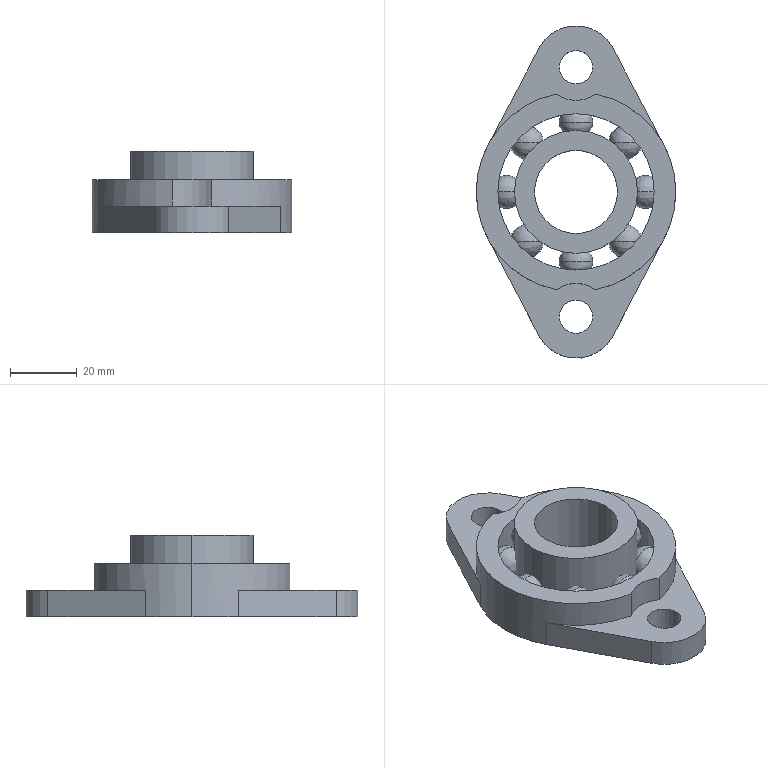Part | STEP file | KFL005 | 10 solids | 43 faces | box 60 x 100 x 24.5 mm | volume 44047 mm3 | cylinder 17 | spline 16 | plane 10 | commonest cylinder face diameters 10 x4 25 x4 60 x3 20 x2 37 x2 47 x2
STEP:
#1=CARTESIAN_POINT('',(-9.849,-14.849,10.));
#2=VERTEX_POINT('',#1);
#3=CARTESIAN_POINT('',(-19.849,-14.849,10.));
#4=VERTEX_POINT('',#3);
#5=CARTESIAN_POINT('',(-14.849,-14.849,10.));
#6=DIRECTION('',(0.,1.,0.));
#7=DIRECTION('',(1.,0.,0.));
#8=AXIS2_PLACEMENT_3D('',#5,#6,#7);
#9=CIRCLE('',#8,5.);
#10=EDGE_CURVE('',#2,#4,#9,.T.);
#11=ORIENTED_EDGE('',*,*,#10,.F.);
#12=CARTESIAN_POINT('',(-14.849,-14.849,10.));
#13=DIRECTION('',(0.,-1.,0.));
#14=DIRECTION('',(1.,0.,0.));
#15=AXIS2_PLACEMENT_3D('',#12,#13,#14);
#16=CIRCLE('',#15,5.);
#17=EDGE_CURVE('',#2,#4,#16,.T.);
#18=ORIENTED_EDGE('',*,*,#17,.T.);
#19=EDGE_LOOP('',(#11,#18));
#20=FACE_OUTER_BOUND('',#19,.T.);
#21=CARTESIAN_POINT('',(-9.849,-14.849,10.));
#22=CARTESIAN_POINT('',(-9.849,-14.849,10.));
#23=CARTESIAN_POINT('',(-9.849,-14.849,10.));
#24=CARTESIAN_POINT('',(-9.849,-14.849,10.));
#25=CARTESIAN_POINT('',(-9.849,-14.849,20.));
#26=CARTESIAN_POINT('',(-9.849,-34.849,20.));
#27=CARTESIAN_POINT('',(-9.849,-34.849,0.));
#28=CARTESIAN_POINT('',(-9.849,-14.849,0.));
#29=CARTESIAN_POINT('',(-19.849,-14.849,20.));
#30=CARTESIAN_POINT('',(-19.849,-34.849,20.));
#31=CARTESIAN_POINT('',(-19.849,-34.849,0.));
#32=CARTESIAN_POINT('',(-19.849,-14.849,0.));
#33=CARTESIAN_POINT('',(-19.849,-14.849,10.));
#34=CARTESIAN_POINT('',(-19.849,-14.849,10.));
#35=CARTESIAN_POINT('',(-19.849,-14.849,10.));
#36=CARTESIAN_POINT('',(-19.849,-14.849,10.));
#37=(BOUNDED_SURFACE()B_SPLINE_SURFACE(3,3,((#21,#22,#23,#24),(#25,#26,#27,#28),(#29,#30,#31,#32),(#33,#34,#35,#36)),.UNSPECIFIED.,.F.,.F.,.T.)B_SPLINE_SURFACE_WITH_KNOTS((4,4),(4,4),(0.,1.),(0.,1.),.UNSPECIFIED.)GEOMETRIC_REPRESENTATION_ITEM()RATIONAL_B_SPLINE_SURFACE(((1.,0.3333,0.3333,1.),(0.3333,0.1111,0.1111,0.3333),(0.3333,0.1111,0.1111,0.3333),(1.,0.3333,0.3333,1.)))REPRESENTATION_ITEM('')SURFACE());
#38=ADVANCED_FACE('',(#20),#37,.T.);
#39=ORIENTED_EDGE('',*,*,#17,.F.);
#40=ORIENTED_EDGE('',*,*,#10,.T.);
#41=EDGE_LOOP('',(#39,#40));
#42=FACE_OUTER_BOUND('',#41,.T.);
#43=CARTESIAN_POINT('',(-9.849,-14.849,10.));
#44=CARTESIAN_POINT('',(-9.849,-14.849,10.));
#45=CARTESIAN_POINT('',(-9.849,-14.849,10.));
#46=CARTESIAN_POINT('',(-9.849,-14.849,10.));
#47=CARTESIAN_POINT('',(-9.849,-14.849,0.));
#48=CARTESIAN_POINT('',(-9.849,5.151,0.));
#49=CARTESIAN_POINT('',(-9.849,5.151,20.));
#50=CARTESIAN_POINT('',(-9.849,-14.849,20.));
#51=CARTESIAN_POINT('',(-19.849,-14.849,0.));
#52=CARTESIAN_POINT('',(-19.849,5.151,0.));
#53=CARTESIAN_POINT('',(-19.849,5.151,20.));
#54=CARTESIAN_POINT('',(-19.849,-14.849,20.));
#55=CARTESIAN_POINT('',(-19.849,-14.849,10.));
#56=CARTESIAN_POINT('',(-19.849,-14.849,10.));
#57=CARTESIAN_POINT('',(-19.849,-14.849,10.));
#58=CARTESIAN_POINT('',(-19.849,-14.849,10.));
#59=(BOUNDED_SURFACE()B_SPLINE_SURFACE(3,3,((#43,#44,#45,#46),(#47,#48,#49,#50),(#51,#52,#53,#54),(#55,#56,#57,#58)),.UNSPECIFIED.,.F.,.F.,.F.)B_SPLINE_SURFACE_WITH_KNOTS((4,4),(4,4),(0.,1.),(0.,1.),.UNSPECIFIED.)GEOMETRIC_REPRESENTATION_ITEM()RATIONAL_B_SPLINE_SURFACE(((1.,0.3333,0.3333,1.),(0.3333,0.1111,0.1111,0.3333),(0.3333,0.1111,0.1111,0.3333),(1.,0.3333,0.3333,1.)))REPRESENTATION_ITEM('')SURFACE());
#60=ADVANCED_FACE('',(#42),#59,.T.);
#61=CLOSED_SHELL('',(#38,#60));
#62=MANIFOLD_SOLID_BREP('',#61);
#63=CARTESIAN_POINT('',(5.,21.,10.));
#64=VERTEX_POINT('',#63);
#65=CARTESIAN_POINT('',(-5.,21.,10.));
#66=VERTEX_POINT('',#65);
#67=CARTESIAN_POINT('',(0.,21.,10.));
#68=DIRECTION('',(0.,1.,0.));
#69=DIRECTION('',(1.,0.,0.));
#70=AXIS2_PLACEMENT_3D('',#67,#68,#69);
#71=CIRCLE('',#70,5.);
#72=EDGE_CURVE('',#64,#66,#71,.T.);
#73=ORIENTED_EDGE('',*,*,#72,.F.);
#74=CARTESIAN_POINT('',(0.,21.,10.));
#75=DIRECTION('',(0.,-1.,0.));
#76=DIRECTION('',(1.,0.,0.));
#77=AXIS2_PLACEMENT_3D('',#74,#75,#76);
#78=CIRCLE('',#77,5.);
#79=EDGE_CURVE('',#64,#66,#78,.T.);
#80=ORIENTED_EDGE('',*,*,#79,.T.);
#81=EDGE_LOOP('',(#73,#80));
#82=FACE_OUTER_BOUND('',#81,.T.);
#83=CARTESIAN_POINT('',(5.,21.,10.));
#84=CARTESIAN_POINT('',(5.,21.,10.));
#85=CARTESIAN_POINT('',(5.,21.,10.));
#86=CARTESIAN_POINT('',(5.,21.,10.));
#87=CARTESIAN_POINT('',(5.,21.,20.));
#88=CARTESIAN_POINT('',(5.,1.,20.));
#89=CARTESIAN_POINT('',(5.,1.,0.));
#90=CARTESIAN_POINT('',(5.,21.,0.));
#91=CARTESIAN_POINT('',(-5.,21.,20.));
#92=CARTESIAN_POINT('',(-5.,1.,20.));
#93=CARTESIAN_POINT('',(-5.,1.,0.));
#94=CARTESIAN_POINT('',(-5.,21.,0.));
#95=CARTESIAN_POINT('',(-5.,21.,10.));
#96=CARTESIAN_POINT('',(-5.,21.,10.));
#97=CARTESIAN_POINT('',(-5.,21.,10.));
#98=CARTESIAN_POINT('',(-5.,21.,10.));
#99=(BOUNDED_SURFACE()B_SPLINE_SURFACE(3,3,((#83,#84,#85,#86),(#87,#88,#89,#90),(#91,#92,#93,#94),(#95,#96,#97,#98)),.UNSPECIFIED.,.F.,.F.,.F.)B_SPLINE_SURFACE_WITH_KNOTS((4,4),(4,4),(0.,1.),(0.,1.),.UNSPECIFIED.)GEOMETRIC_REPRESENTATION_ITEM()RATIONAL_B_SPLINE_SURFACE(((1.,0.3333,0.3333,1.),(0.3333,0.1111,0.1111,0.3333),(0.3333,0.1111,0.1111,0.3333),(1.,0.3333,0.3333,1.)))REPRESENTATION_ITEM('')SURFACE());
#100=ADVANCED_FACE('',(#82),#99,.T.);
#101=ORIENTED_EDGE('',*,*,#79,.F.);
#102=ORIENTED_EDGE('',*,*,#72,.T.);
#103=EDGE_LOOP('',(#101,#102));
#104=FACE_OUTER_BOUND('',#103,.T.);
#105=CARTESIAN_POINT('',(5.,21.,10.));
#106=CARTESIAN_POINT('',(5.,21.,10.));
#107=CARTESIAN_POINT('',(5.,21.,10.));
#108=CARTESIAN_POINT('',(5.,21.,10.));
#109=CARTESIAN_POINT('',(5.,21.,0.));
#110=CARTESIAN_POINT('',(5.,41.,0.));
#111=CARTESIAN_POINT('',(5.,41.,20.));
#112=CARTESIAN_POINT('',(5.,21.,20.));
#113=CARTESIAN_POINT('',(-5.,21.,0.));
#114=CARTESIAN_POINT('',(-5.,41.,0.));
#115=CARTESIAN_POINT('',(-5.,41.,20.));
#116=CARTESIAN_POINT('',(-5.,21.,20.));
#117=CARTESIAN_POINT('',(-5.,21.,10.));
#118=CARTESIAN_POINT('',(-5.,21.,10.));
#119=CARTESIAN_POINT('',(-5.,21.,10.));
#120=CARTESIAN_POINT('',(-5.,21.,10.));
#121=(BOUNDED_SURFACE()B_SPLINE_SURFACE(3,3,((#105,#106,#107,#108),(#109,#110,#111,#112),(#113,#114,#115,#116),(#117,#118,#119,#120)),.UNSPECIFIED.,.F.,.F.,.F.)B_SPLINE_SURFACE_WITH_KNOTS((4,4),(4,4),(0.,1.),(0.,1.),.UNSPECIFIED.)GEOMETRIC_REPRESENTATION_ITEM()RATIONAL_B_SPLINE_SURFACE(((1.,0.3333,0.3333,1.),(0.3333,0.1111,0.1111,0.3333),(0.3333,0.1111,0.1111,0.3333),(1.,0.3333,0.3333,1.)))REPRESENTATION_ITEM('')SURFACE());
#122=ADVANCED_FACE('',(#104),#121,.T.);
#123=CLOSED_SHELL('',(#100,#122));
#124=MANIFOLD_SOLID_BREP('',#123);
#125=CARTESIAN_POINT('',(5.,37.5,8.));
#126=VERTEX_POINT('',#125);
#127=CARTESIAN_POINT('',(-5.,37.5,8.));
#128=VERTEX_POINT('',#127);
#129=CARTESIAN_POINT('',(0.,37.5,8.));
#130=DIRECTION('',(0.,0.,-1.));
#131=DIRECTION('',(-1.,0.,0.));
#132=AXIS2_PLACEMENT_3D('',#129,#130,#131);
#133=CIRCLE('',#132,5.);
#134=EDGE_CURVE('',#126,#128,#133,.T.);
#135=ORIENTED_EDGE('',*,*,#134,.F.);
#136=CARTESIAN_POINT('',(5.,37.5,0.));
#137=VERTEX_POINT('',#136);
#138=CARTESIAN_POINT('',(5.,37.5,8.));
#139=DIRECTION('',(0.,0.,-1.));
#140=VECTOR('',#139,1000.);
#141=LINE('',#138,#140);
#142=EDGE_CURVE('',#126,#137,#141,.T.);
#143=ORIENTED_EDGE('',*,*,#142,.T.);
#144=CARTESIAN_POINT('',(-5.,37.5,0.));
#145=VERTEX_POINT('',#144);
#146=CARTESIAN_POINT('',(0.,37.5,0.));
#147=DIRECTION('',(0.,0.,-1.));
#148=DIRECTION('',(-1.,0.,0.));
#149=AXIS2_PLACEMENT_3D('',#146,#147,#148);
#150=CIRCLE('',#149,5.);
#151=EDGE_CURVE('',#137,#145,#150,.T.);
#152=ORIENTED_EDGE('',*,*,#151,.T.);
#153=CARTESIAN_POINT('',(-5.,37.5,8.));
#154=DIRECTION('',(0.,0.,-1.));
#155=VECTOR('',#154,1000.);
#156=LINE('',#153,#155);
#157=EDGE_CURVE('',#128,#145,#156,.T.);
#158=ORIENTED_EDGE('',*,*,#157,.F.);
#159=EDGE_LOOP('',(#135,#143,#152,#158));
#160=FACE_OUTER_BOUND('',#159,.T.);
#161=CARTESIAN_POINT('',(0.,37.5,8.));
#162=DIRECTION('',(0.,0.,-1.));
#163=DIRECTION('',(-1.,0.,0.));
#164=AXIS2_PLACEMENT_3D('',#161,#162,#163);
#165=CYLINDRICAL_SURFACE('',#164,5.);
#166=ADVANCED_FACE('',(#160),#165,.F.);
#167=CARTESIAN_POINT('',(23.5,0.,16.));
#168=VERTEX_POINT('',#167);
#169=CARTESIAN_POINT('',(-23.5,0.,16.));
#170=VERTEX_POINT('',#169);
#171=CARTESIAN_POINT('',(0.,0.,16.));
#172=DIRECTION('',(0.,0.,-1.));
#173=DIRECTION('',(-1.,0.,0.));
#174=AXIS2_PLACEMENT_3D('',#171,#172,#173);
#175=CIRCLE('',#174,23.5);
#176=EDGE_CURVE('',#168,#170,#175,.T.);
#177=ORIENTED_EDGE('',*,*,#176,.F.);
#178=CARTESIAN_POINT('',(23.5,0.,0.));
#179=VERTEX_POINT('',#178);
#180=CARTESIAN_POINT('',(23.5,0.,8.));
#181=DIRECTION('',(0.,0.,-1.));
#182=VECTOR('',#181,1000.);
#183=LINE('',#180,#182);
#184=EDGE_CURVE('',#168,#179,#183,.T.);
#185=ORIENTED_EDGE('',*,*,#184,.T.);
#186=CARTESIAN_POINT('',(-23.5,0.,0.));
#187=VERTEX_POINT('',#186);
#188=CARTESIAN_POINT('',(0.,0.,0.));
#189=DIRECTION('',(0.,0.,-1.));
#190=DIRECTION('',(-1.,0.,0.));
#191=AXIS2_PLACEMENT_3D('',#188,#189,#190);
#192=CIRCLE('',#191,23.5);
#193=EDGE_CURVE('',#179,#187,#192,.T.);
#194=ORIENTED_EDGE('',*,*,#193,.T.);
#195=CARTESIAN_POINT('',(-23.5,0.,8.));
#196=DIRECTION('',(0.,0.,-1.));
#197=VECTOR('',#196,1000.);
#198=LINE('',#195,#197);
#199=EDGE_CURVE('',#170,#187,#198,.T.);
#200=ORIENTED_EDGE('',*,*,#199,.F.);
#201=EDGE_LOOP('',(#177,#185,#194,#200));
#202=FACE_OUTER_BOUND('',#201,.T.);
#203=CARTESIAN_POINT('',(0.,0.,8.));
#204=DIRECTION('',(0.,0.,-1.));
#205=DIRECTION('',(-1.,0.,0.));
#206=AXIS2_PLACEMENT_3D('',#203,#204,#205);
#207=CYLINDRICAL_SURFACE('',#206,23.5);
#208=ADVANCED_FACE('',(#202),#207,.F.);
#209=CARTESIAN_POINT('',(5.,-37.5,8.));
#210=VERTEX_POINT('',#209);
#211=CARTESIAN_POINT('',(-5.,-37.5,8.));
#212=VERTEX_POINT('',#211);
#213=CARTESIAN_POINT('',(0.,-37.5,8.));
#214=DIRECTION('',(0.,0.,-1.));
#215=DIRECTION('',(-1.,0.,0.));
#216=AXIS2_PLACEMENT_3D('',#213,#214,#215);
#217=CIRCLE('',#216,5.);
#218=EDGE_CURVE('',#210,#212,#217,.T.);
#219=ORIENTED_EDGE('',*,*,#218,.F.);
#220=CARTESIAN_POINT('',(5.,-37.5,0.));
#221=VERTEX_POINT('',#220);
#222=CARTESIAN_POINT('',(5.,-37.5,8.));
#223=DIRECTION('',(0.,0.,-1.));
#224=VECTOR('',#223,1000.);
#225=LINE('',#222,#224);
#226=EDGE_CURVE('',#210,#221,#225,.T.);
#227=ORIENTED_EDGE('',*,*,#226,.T.);
#228=CARTESIAN_POINT('',(-5.,-37.5,0.));
#229=VERTEX_POINT('',#228);
#230=CARTESIAN_POINT('',(0.,-37.5,0.));
#231=DIRECTION('',(0.,0.,-1.));
#232=DIRECTION('',(-1.,0.,0.));
#233=AXIS2_PLACEMENT_3D('',#230,#231,#232);
#234=CIRCLE('',#233,5.);
#235=EDGE_CURVE('',#221,#229,#234,.T.);
#236=ORIENTED_EDGE('',*,*,#235,.T.);
#237=CARTESIAN_POINT('',(-5.,-37.5,8.));
#238=DIRECTION('',(0.,0.,-1.));
#239=VECTOR('',#238,1000.);
#240=LINE('',#237,#239);
#241=EDGE_CURVE('',#212,#229,#240,.T.);
#242=ORIENTED_EDGE('',*,*,#241,.F.);
#243=EDGE_LOOP('',(#219,#227,#236,#242));
#244=FACE_OUTER_BOUND('',#243,.T.);
#245=CARTESIAN_POINT('',(0.,-37.5,8.));
#246=DIRECTION('',(0.,0.,-1.));
#247=DIRECTION('',(-1.,0.,0.));
#248=AXIS2_PLACEMENT_3D('',#245,#246,#247);
#249=CYLINDRICAL_SURFACE('',#248,5.);
#250=ADVANCED_FACE('',(#244),#249,.F.);
#251=CARTESIAN_POINT('',(-5.887,-29.417,16.));
#252=VERTEX_POINT('',#251);
#253=CARTESIAN_POINT('',(-30.,0.,16.));
#254=VERTEX_POINT('',#253);
#255=CARTESIAN_POINT('',(0.,0.,16.));
#256=DIRECTION('',(0.,0.,-1.));
#257=DIRECTION('',(-1.,0.,0.));
#258=AXIS2_PLACEMENT_3D('',#255,#256,#257);
#259=CIRCLE('',#258,30.);
#260=EDGE_CURVE('',#252,#254,#259,.T.);
#261=ORIENTED_EDGE('',*,*,#260,.T.);
#262=CARTESIAN_POINT('',(-30.,0.,0.));
#263=VERTEX_POINT('',#262);
#264=CARTESIAN_POINT('',(-30.,0.,8.));
#265=DIRECTION('',(0.,0.,-1.));
#266=VECTOR('',#265,1000.);
#267=LINE('',#264,#266);
#268=EDGE_CURVE('',#254,#263,#267,.T.);
#269=ORIENTED_EDGE('',*,*,#268,.T.);
#270=CARTESIAN_POINT('',(-26.533,-14.,0.));
#271=VERTEX_POINT('',#270);
#272=CARTESIAN_POINT('',(0.,0.,0.));
#273=DIRECTION('',(0.,0.,1.));
#274=DIRECTION('',(-1.,0.,0.));
#275=AXIS2_PLACEMENT_3D('',#272,#273,#274);
#276=CIRCLE('',#275,30.);
#277=EDGE_CURVE('',#263,#271,#276,.T.);
#278=ORIENTED_EDGE('',*,*,#277,.T.);
#279=CARTESIAN_POINT('',(-26.533,-14.,8.));
#280=VERTEX_POINT('',#279);
#281=CARTESIAN_POINT('',(-26.533,-14.,8.));
#282=DIRECTION('',(0.,0.,1.));
#283=VECTOR('',#282,1000.);
#284=LINE('',#281,#283);
#285=EDGE_CURVE('',#271,#280,#284,.T.);
#286=ORIENTED_EDGE('',*,*,#285,.T.);
#287=CARTESIAN_POINT('',(-5.887,-29.417,8.));
#288=VERTEX_POINT('',#287);
#289=CARTESIAN_POINT('',(0.,0.,8.));
#290=DIRECTION('',(0.,0.,1.));
#291=DIRECTION('',(-1.,0.,0.));
#292=AXIS2_PLACEMENT_3D('',#289,#290,#291);
#293=CIRCLE('',#292,30.);
#294=EDGE_CURVE('',#280,#288,#293,.T.);
#295=ORIENTED_EDGE('',*,*,#294,.T.);
#296=CARTESIAN_POINT('',(-5.887,-29.417,8.));
#297=DIRECTION('',(0.,0.,1.));
#298=VECTOR('',#297,1000.);
#299=LINE('',#296,#298);
#300=EDGE_CURVE('',#288,#252,#299,.T.);
#301=ORIENTED_EDGE('',*,*,#300,.T.);
#302=EDGE_LOOP('',(#261,#269,#278,#286,#295,#301));
#303=FACE_OUTER_BOUND('',#302,.T.);
#304=CARTESIAN_POINT('',(0.,0.,8.));
#305=DIRECTION('',(0.,0.,-1.));
#306=DIRECTION('',(-1.,0.,0.));
#307=AXIS2_PLACEMENT_3D('',#304,#305,#306);
#308=CYLINDRICAL_SURFACE('',#307,30.);
#309=ADVANCED_FACE('',(#303),#308,.T.);
#310=CARTESIAN_POINT('',(0.,37.5,0.));
#311=DIRECTION('',(0.,0.,-1.));
#312=DIRECTION('',(-1.,0.,0.));
#313=AXIS2_PLACEMENT_3D('',#310,#311,#312);
#314=CIRCLE('',#313,5.);
#315=EDGE_CURVE('',#145,#137,#314,.T.);
#316=ORIENTED_EDGE('',*,*,#315,.F.);
#317=ORIENTED_EDGE('',*,*,#151,.F.);
#318=EDGE_LOOP('',(#316,#317));
#319=FACE_BOUND('',#318,.T.);
#320=CARTESIAN_POINT('',(0.,0.,0.));
#321=DIRECTION('',(0.,0.,-1.));
#322=DIRECTION('',(-1.,0.,0.));
#323=AXIS2_PLACEMENT_3D('',#320,#321,#322);
#324=CIRCLE('',#323,23.5);
#325=EDGE_CURVE('',#187,#179,#324,.T.);
#326=ORIENTED_EDGE('',*,*,#325,.F.);
#327=ORIENTED_EDGE('',*,*,#193,.F.);
#328=EDGE_LOOP('',(#326,#327));
#329=FACE_BOUND('',#328,.T.);
#330=CARTESIAN_POINT('',(0.,-37.5,0.));
#331=DIRECTION('',(0.,0.,-1.));
#332=DIRECTION('',(-1.,0.,0.));
#333=AXIS2_PLACEMENT_3D('',#330,#331,#332);
#334=CIRCLE('',#333,5.);
#335=EDGE_CURVE('',#229,#221,#334,.T.);
#336=ORIENTED_EDGE('',*,*,#335,.F.);
#337=ORIENTED_EDGE('',*,*,#235,.F.);
#338=EDGE_LOOP('',(#336,#337));
#339=FACE_BOUND('',#338,.T.);
#340=CARTESIAN_POINT('',(-11.055,43.333,0.));
#341=VERTEX_POINT('',#340);
#342=CARTESIAN_POINT('',(-26.533,14.,0.));
#343=VERTEX_POINT('',#342);
#344=CARTESIAN_POINT('',(-11.055,43.333,0.));
#345=DIRECTION('',(-0.4667,-0.8844,0.));
#346=VECTOR('',#345,1000.);
#347=LINE('',#344,#346);
#348=EDGE_CURVE('',#341,#343,#347,.T.);
#349=ORIENTED_EDGE('',*,*,#348,.F.);
#350=CARTESIAN_POINT('',(11.055,43.333,0.));
#351=VERTEX_POINT('',#350);
#352=CARTESIAN_POINT('',(0.,37.5,0.));
#353=DIRECTION('',(0.,0.,1.));
#354=DIRECTION('',(-1.,0.,0.));
#355=AXIS2_PLACEMENT_3D('',#352,#353,#354);
#356=CIRCLE('',#355,12.5);
#357=EDGE_CURVE('',#351,#341,#356,.T.);
#358=ORIENTED_EDGE('',*,*,#357,.F.);
#359=CARTESIAN_POINT('',(26.533,14.,0.));
#360=VERTEX_POINT('',#359);
#361=CARTESIAN_POINT('',(26.533,14.,0.));
#362=DIRECTION('',(-0.4667,0.8844,0.));
#363=VECTOR('',#362,1000.);
#364=LINE('',#361,#363);
#365=EDGE_CURVE('',#360,#351,#364,.T.);
#366=ORIENTED_EDGE('',*,*,#365,.F.);
#367=CARTESIAN_POINT('',(26.533,-14.,0.));
#368=VERTEX_POINT('',#367);
#369=CARTESIAN_POINT('',(0.,0.,0.));
#370=DIRECTION('',(0.,0.,1.));
#371=DIRECTION('',(-1.,0.,0.));
#372=AXIS2_PLACEMENT_3D('',#369,#370,#371);
#373=CIRCLE('',#372,30.);
#374=EDGE_CURVE('',#368,#360,#373,.T.);
#375=ORIENTED_EDGE('',*,*,#374,.F.);
#376=CARTESIAN_POINT('',(11.055,-43.333,0.));
#377=VERTEX_POINT('',#376);
#378=CARTESIAN_POINT('',(11.055,-43.333,0.));
#379=DIRECTION('',(0.4667,0.8844,0.));
#380=VECTOR('',#379,1000.);
#381=LINE('',#378,#380);
#382=EDGE_CURVE('',#377,#368,#381,.T.);
#383=ORIENTED_EDGE('',*,*,#382,.F.);
#384=CARTESIAN_POINT('',(-11.055,-43.333,0.));
#385=VERTEX_POINT('',#384);
#386=CARTESIAN_POINT('',(0.,-37.5,0.));
#387=DIRECTION('',(0.,0.,1.));
#388=DIRECTION('',(-1.,0.,0.));
#389=AXIS2_PLACEMENT_3D('',#386,#387,#388);
#390=CIRCLE('',#389,12.5);
#391=EDGE_CURVE('',#385,#377,#390,.T.);
#392=ORIENTED_EDGE('',*,*,#391,.F.);
#393=CARTESIAN_POINT('',(-26.533,-14.,0.));
#394=DIRECTION('',(0.4667,-0.8844,0.));
#395=VECTOR('',#394,1000.);
#396=LINE('',#393,#395);
#397=EDGE_CURVE('',#271,#385,#396,.T.);
#398=ORIENTED_EDGE('',*,*,#397,.F.);
#399=ORIENTED_EDGE('',*,*,#277,.F.);
#400=CARTESIAN_POINT('',(0.,0.,0.));
#401=DIRECTION('',(0.,0.,1.));
#402=DIRECTION('',(-1.,0.,0.));
#403=AXIS2_PLACEMENT_3D('',#400,#401,#402);
#404=CIRCLE('',#403,30.);
#405=EDGE_CURVE('',#343,#263,#404,.T.);
#406=ORIENTED_EDGE('',*,*,#405,.F.);
#407=EDGE_LOOP('',(#349,#358,#366,#375,#383,#392,#398,#399,#406));
#408=FACE_OUTER_BOUND('',#407,.T.);
#409=CARTESIAN_POINT('',(0.,0.,0.));
#410=DIRECTION('',(0.,0.,1.));
#411=DIRECTION('',(1.,0.,0.));
#412=AXIS2_PLACEMENT_3D('',#409,#410,#411);
#413=PLANE('',#412);
#414=ADVANCED_FACE('',(#319,#329,#339,#408),#413,.F.);
#415=ORIENTED_EDGE('',*,*,#142,.F.);
#416=CARTESIAN_POINT('',(0.,37.5,8.));
#417=DIRECTION('',(0.,0.,-1.));
#418=DIRECTION('',(-1.,0.,0.));
#419=AXIS2_PLACEMENT_3D('',#416,#417,#418);
#420=CIRCLE('',#419,5.);
#421=EDGE_CURVE('',#128,#126,#420,.T.);
#422=ORIENTED_EDGE('',*,*,#421,.F.);
#423=ORIENTED_EDGE('',*,*,#157,.T.);
#424=ORIENTED_EDGE('',*,*,#315,.T.);
#425=EDGE_LOOP('',(#415,#422,#423,#424));
#426=FACE_OUTER_BOUND('',#425,.T.);
#427=CARTESIAN_POINT('',(0.,37.5,8.));
#428=DIRECTION('',(0.,0.,-1.));
#429=DIRECTION('',(-1.,0.,0.));
#430=AXIS2_PLACEMENT_3D('',#427,#428,#429);
#431=CYLINDRICAL_SURFACE('',#430,5.);
#432=ADVANCED_FACE('',(#426),#431,.F.);
#433=ORIENTED_EDGE('',*,*,#184,.F.);
#434=CARTESIAN_POINT('',(0.,0.,16.));
#435=DIRECTION('',(0.,0.,-1.));
#436=DIRECTION('',(-1.,0.,0.));
#437=AXIS2_PLACEMENT_3D('',#434,#435,#436);
#438=CIRCLE('',#437,23.5);
#439=EDGE_CURVE('',#170,#168,#438,.T.);
#440=ORIENTED_EDGE('',*,*,#439,.F.);
#441=ORIENTED_EDGE('',*,*,#199,.T.);
#442=ORIENTED_EDGE('',*,*,#325,.T.);
#443=EDGE_LOOP('',(#433,#440,#441,#442));
#444=FACE_OUTER_BOUND('',#443,.T.);
#445=CARTESIAN_POINT('',(0.,0.,8.));
#446=DIRECTION('',(0.,0.,-1.));
#447=DIRECTION('',(-1.,0.,0.));
#448=AXIS2_PLACEMENT_3D('',#445,#446,#447);
#449=CYLINDRICAL_SURFACE('',#448,23.5);
#450=ADVANCED_FACE('',(#444),#449,.F.);
#451=ORIENTED_EDGE('',*,*,#226,.F.);
#452=CARTESIAN_POINT('',(0.,-37.5,8.));
#453=DIRECTION('',(0.,0.,-1.));
#454=DIRECTION('',(-1.,0.,0.));
#455=AXIS2_PLACEMENT_3D('',#452,#453,#454);
#456=CIRCLE('',#455,5.);
#457=EDGE_CURVE('',#212,#210,#456,.T.);
#458=ORIENTED_EDGE('',*,*,#457,.F.);
#459=ORIENTED_EDGE('',*,*,#241,.T.);
#460=ORIENTED_EDGE('',*,*,#335,.T.);
#461=EDGE_LOOP('',(#451,#458,#459,#460));
#462=FACE_OUTER_BOUND('',#461,.T.);
#463=CARTESIAN_POINT('',(0.,-37.5,8.));
#464=DIRECTION('',(0.,0.,-1.));
#465=DIRECTION('',(-1.,0.,0.));
#466=AXIS2_PLACEMENT_3D('',#463,#464,#465);
#467=CYLINDRICAL_SURFACE('',#466,5.);
#468=ADVANCED_FACE('',(#462),#467,.F.);
#469=ORIENTED_EDGE('',*,*,#268,.F.);
#470=CARTESIAN_POINT('',(-5.887,29.417,16.));
#471=VERTEX_POINT('',#470);
#472=CARTESIAN_POINT('',(0.,0.,16.));
#473=DIRECTION('',(0.,0.,-1.));
#474=DIRECTION('',(-1.,0.,0.));
#475=AXIS2_PLACEMENT_3D('',#472,#473,#474);
#476=CIRCLE('',#475,30.);
#477=EDGE_CURVE('',#254,#471,#476,.T.);
#478=ORIENTED_EDGE('',*,*,#477,.T.);
#479=CARTESIAN_POINT('',(-5.887,29.417,8.));
#480=VERTEX_POINT('',#479);
#481=CARTESIAN_POINT('',(-5.887,29.417,8.));
#482=DIRECTION('',(0.,0.,-1.));
#483=VECTOR('',#482,1000.);
#484=LINE('',#481,#483);
#485=EDGE_CURVE('',#471,#480,#484,.T.);
#486=ORIENTED_EDGE('',*,*,#485,.T.);
#487=CARTESIAN_POINT('',(-26.533,14.,8.));
#488=VERTEX_POINT('',#487);
#489=CARTESIAN_POINT('',(0.,0.,8.));
#490=DIRECTION('',(0.,0.,1.));
#491=DIRECTION('',(-1.,0.,0.));
#492=AXIS2_PLACEMENT_3D('',#489,#490,#491);
#493=CIRCLE('',#492,30.);
#494=EDGE_CURVE('',#480,#488,#493,.T.);
#495=ORIENTED_EDGE('',*,*,#494,.T.);
#496=CARTESIAN_POINT('',(-26.533,14.,8.));
#497=DIRECTION('',(0.,0.,-1.));
#498=VECTOR('',#497,1000.);
#499=LINE('',#496,#498);
#500=EDGE_CURVE('',#488,#343,#499,.T.);
#501=ORIENTED_EDGE('',*,*,#500,.T.);
#502=ORIENTED_EDGE('',*,*,#405,.T.);
#503=EDGE_LOOP('',(#469,#478,#486,#495,#501,#502));
#504=FACE_OUTER_BOUND('',#503,.T.);
#505=CARTESIAN_POINT('',(0.,0.,8.));
#506=DIRECTION('',(0.,0.,-1.));
#507=DIRECTION('',(-1.,0.,0.));
#508=AXIS2_PLACEMENT_3D('',#505,#506,#507);
#509=CYLINDRICAL_SURFACE('',#508,30.);
#510=ADVANCED_FACE('',(#504),#509,.T.);
#511=ORIENTED_EDGE('',*,*,#500,.F.);
#512=CARTESIAN_POINT('',(-11.055,43.333,8.));
#513=VERTEX_POINT('',#512);
#514=CARTESIAN_POINT('',(-11.055,43.333,8.));
#515=DIRECTION('',(-0.4667,-0.8844,0.));
#516=VECTOR('',#515,1000.);
#517=LINE('',#514,#516);
#518=EDGE_CURVE('',#513,#488,#517,.T.);
#519=ORIENTED_EDGE('',*,*,#518,.F.);
#520=CARTESIAN_POINT('',(-11.055,43.333,8.));
#521=DIRECTION('',(0.,0.,1.));
#522=VECTOR('',#521,1000.);
#523=LINE('',#520,#522);
#524=EDGE_CURVE('',#341,#513,#523,.T.);
#525=ORIENTED_EDGE('',*,*,#524,.F.);
#526=ORIENTED_EDGE('',*,*,#348,.T.);
#527=EDGE_LOOP('',(#511,#519,#525,#526));
#528=FACE_OUTER_BOUND('',#527,.T.);
#529=CARTESIAN_POINT('',(-11.055,43.333,8.));
#530=DIRECTION('',(0.8844,-0.4667,0.));
#531=DIRECTION('',(0.4667,0.8844,0.));
#532=AXIS2_PLACEMENT_3D('',#529,#530,#531);
#533=PLANE('',#532);
#534=ADVANCED_FACE('',(#528),#533,.F.);
#535=CARTESIAN_POINT('',(11.055,43.333,8.));
#536=VERTEX_POINT('',#535);
#537=CARTESIAN_POINT('',(0.,37.5,8.));
#538=DIRECTION('',(0.,0.,-1.));
#539=DIRECTION('',(-1.,0.,0.));
#540=AXIS2_PLACEMENT_3D('',#537,#538,#539);
#541=CIRCLE('',#540,12.5);
#542=EDGE_CURVE('',#513,#536,#541,.T.);
#543=ORIENTED_EDGE('',*,*,#542,.T.);
#544=CARTESIAN_POINT('',(11.055,43.333,8.));
#545=DIRECTION('',(0.,0.,-1.));
#546=VECTOR('',#545,1000.);
#547=LINE('',#544,#546);
#548=EDGE_CURVE('',#536,#351,#547,.T.);
#549=ORIENTED_EDGE('',*,*,#548,.T.);
#550=ORIENTED_EDGE('',*,*,#357,.T.);
#551=ORIENTED_EDGE('',*,*,#524,.T.);
#552=EDGE_LOOP('',(#543,#549,#550,#551));
#553=FACE_OUTER_BOUND('',#552,.T.);
#554=CARTESIAN_POINT('',(0.,37.5,8.));
#555=DIRECTION('',(0.,0.,-1.));
#556=DIRECTION('',(-1.,0.,0.));
#557=AXIS2_PLACEMENT_3D('',#554,#555,#556);
#558=CYLINDRICAL_SURFACE('',#557,12.5);
#559=ADVANCED_FACE('',(#553),#558,.T.);
#560=ORIENTED_EDGE('',*,*,#548,.F.);
#561=CARTESIAN_POINT('',(26.533,14.,8.));
#562=VERTEX_POINT('',#561);
#563=CARTESIAN_POINT('',(26.533,14.,8.));
#564=DIRECTION('',(-0.4667,0.8844,0.));
#565=VECTOR('',#564,1000.);
#566=LINE('',#563,#565);
#567=EDGE_CURVE('',#562,#536,#566,.T.);
#568=ORIENTED_EDGE('',*,*,#567,.F.);
#569=CARTESIAN_POINT('',(26.533,14.,8.));
#570=DIRECTION('',(0.,0.,1.));
#571=VECTOR('',#570,1000.);
#572=LINE('',#569,#571);
#573=EDGE_CURVE('',#360,#562,#572,.T.);
#574=ORIENTED_EDGE('',*,*,#573,.F.);
#575=ORIENTED_EDGE('',*,*,#365,.T.);
#576=EDGE_LOOP('',(#560,#568,#574,#575));
#577=FACE_OUTER_BOUND('',#576,.T.);
#578=CARTESIAN_POINT('',(26.533,14.,8.));
#579=DIRECTION('',(-0.8844,-0.4667,0.));
#580=DIRECTION('',(0.4667,-0.8844,0.));
#581=AXIS2_PLACEMENT_3D('',#578,#579,#580);
#582=PLANE('',#581);
#583=ADVANCED_FACE('',(#577),#582,.F.);
#584=CARTESIAN_POINT('',(5.887,-29.417,8.));
#585=VERTEX_POINT('',#584);
#586=CARTESIAN_POINT('',(26.533,-14.,8.));
#587=VERTEX_POINT('',#586);
#588=CARTESIAN_POINT('',(0.,0.,8.));
#589=DIRECTION('',(0.,0.,1.));
#590=DIRECTION('',(-1.,0.,0.));
#591=AXIS2_PLACEMENT_3D('',#588,#589,#590);
#592=CIRCLE('',#591,30.);
#593=EDGE_CURVE('',#585,#587,#592,.T.);
#594=ORIENTED_EDGE('',*,*,#593,.T.);
#595=CARTESIAN_POINT('',(26.533,-14.,8.));
#596=DIRECTION('',(0.,0.,-1.));
#597=VECTOR('',#596,1000.);
#598=LINE('',#595,#597);
#599=EDGE_CURVE('',#587,#368,#598,.T.);
#600=ORIENTED_EDGE('',*,*,#599,.T.);
#601=ORIENTED_EDGE('',*,*,#374,.T.);
#602=ORIENTED_EDGE('',*,*,#573,.T.);
#603=CARTESIAN_POINT('',(5.887,29.417,8.));
#604=VERTEX_POINT('',#603);
#605=CARTESIAN_POINT('',(0.,0.,8.));
#606=DIRECTION('',(0.,0.,1.));
#607=DIRECTION('',(-1.,0.,0.));
#608=AXIS2_PLACEMENT_3D('',#605,#606,#607);
#609=CIRCLE('',#608,30.);
#610=EDGE_CURVE('',#562,#604,#609,.T.);
#611=ORIENTED_EDGE('',*,*,#610,.T.);
#612=CARTESIAN_POINT('',(5.887,29.417,16.));
#613=VERTEX_POINT('',#612);
#614=CARTESIAN_POINT('',(5.887,29.417,8.));
#615=DIRECTION('',(0.,0.,1.));
#616=VECTOR('',#615,1000.);
#617=LINE('',#614,#616);
#618=EDGE_CURVE('',#604,#613,#617,.T.);
#619=ORIENTED_EDGE('',*,*,#618,.T.);
#620=CARTESIAN_POINT('',(5.887,-29.417,16.));
#621=VERTEX_POINT('',#620);
#622=CARTESIAN_POINT('',(0.,0.,16.));
#623=DIRECTION('',(0.,0.,-1.));
#624=DIRECTION('',(-1.,0.,0.));
#625=AXIS2_PLACEMENT_3D('',#622,#623,#624);
#626=CIRCLE('',#625,30.);
#627=EDGE_CURVE('',#613,#621,#626,.T.);
#628=ORIENTED_EDGE('',*,*,#627,.T.);
#629=CARTESIAN_POINT('',(5.887,-29.417,8.));
#630=DIRECTION('',(0.,0.,-1.));
#631=VECTOR('',#630,1000.);
#632=LINE('',#629,#631);
#633=EDGE_CURVE('',#621,#585,#632,.T.);
#634=ORIENTED_EDGE('',*,*,#633,.T.);
#635=EDGE_LOOP('',(#594,#600,#601,#602,#611,#619,#628,#634));
#636=FACE_OUTER_BOUND('',#635,.T.);
#637=CARTESIAN_POINT('',(0.,0.,8.));
#638=DIRECTION('',(0.,0.,-1.));
#639=DIRECTION('',(-1.,0.,0.));
#640=AXIS2_PLACEMENT_3D('',#637,#638,#639);
#641=CYLINDRICAL_SURFACE('',#640,30.);
#642=ADVANCED_FACE('',(#636),#641,.T.);
#643=ORIENTED_EDGE('',*,*,#599,.F.);
#644=CARTESIAN_POINT('',(11.055,-43.333,8.));
#645=VERTEX_POINT('',#644);
#646=CARTESIAN_POINT('',(11.055,-43.333,8.));
#647=DIRECTION('',(0.4667,0.8844,0.));
#648=VECTOR('',#647,1000.);
#649=LINE('',#646,#648);
#650=EDGE_CURVE('',#645,#587,#649,.T.);
#651=ORIENTED_EDGE('',*,*,#650,.F.);
#652=CARTESIAN_POINT('',(11.055,-43.333,8.));
#653=DIRECTION('',(0.,0.,1.));
#654=VECTOR('',#653,1000.);
#655=LINE('',#652,#654);
#656=EDGE_CURVE('',#377,#645,#655,.T.);
#657=ORIENTED_EDGE('',*,*,#656,.F.);
#658=ORIENTED_EDGE('',*,*,#382,.T.);
#659=EDGE_LOOP('',(#643,#651,#657,#658));
#660=FACE_OUTER_BOUND('',#659,.T.);
#661=CARTESIAN_POINT('',(11.055,-43.333,8.));
#662=DIRECTION('',(-0.8844,0.4667,0.));
#663=DIRECTION('',(-0.4667,-0.8844,0.));
#664=AXIS2_PLACEMENT_3D('',#661,#662,#663);
#665=PLANE('',#664);
#666=ADVANCED_FACE('',(#660),#665,.F.);
#667=CARTESIAN_POINT('',(-11.055,-43.333,8.));
#668=VERTEX_POINT('',#667);
#669=CARTESIAN_POINT('',(0.,-37.5,8.));
#670=DIRECTION('',(0.,0.,-1.));
#671=DIRECTION('',(-1.,0.,0.));
#672=AXIS2_PLACEMENT_3D('',#669,#670,#671);
#673=CIRCLE('',#672,12.5);
#674=EDGE_CURVE('',#645,#668,#673,.T.);
#675=ORIENTED_EDGE('',*,*,#674,.T.);
#676=CARTESIAN_POINT('',(-11.055,-43.333,8.));
#677=DIRECTION('',(0.,0.,-1.));
#678=VECTOR('',#677,1000.);
#679=LINE('',#676,#678);
#680=EDGE_CURVE('',#668,#385,#679,.T.);
#681=ORIENTED_EDGE('',*,*,#680,.T.);
#682=ORIENTED_EDGE('',*,*,#391,.T.);
#683=ORIENTED_EDGE('',*,*,#656,.T.);
#684=EDGE_LOOP('',(#675,#681,#682,#683));
#685=FACE_OUTER_BOUND('',#684,.T.);
#686=CARTESIAN_POINT('',(0.,-37.5,8.));
#687=DIRECTION('',(0.,0.,-1.));
#688=DIRECTION('',(-1.,0.,0.));
#689=AXIS2_PLACEMENT_3D('',#686,#687,#688);
#690=CYLINDRICAL_SURFACE('',#689,12.5);
#691=ADVANCED_FACE('',(#685),#690,.T.);
#692=ORIENTED_EDGE('',*,*,#680,.F.);
#693=CARTESIAN_POINT('',(-26.533,-14.,8.));
#694=DIRECTION('',(0.4667,-0.8844,0.));
#695=VECTOR('',#694,1000.);
#696=LINE('',#693,#695);
#697=EDGE_CURVE('',#280,#668,#696,.T.);
#698=ORIENTED_EDGE('',*,*,#697,.F.);
#699=ORIENTED_EDGE('',*,*,#285,.F.);
#700=ORIENTED_EDGE('',*,*,#397,.T.);
#701=EDGE_LOOP('',(#692,#698,#699,#700));
#702=FACE_OUTER_BOUND('',#701,.T.);
#703=CARTESIAN_POINT('',(-26.533,-14.,8.));
#704=DIRECTION('',(0.8844,0.4667,0.));
#705=DIRECTION('',(-0.4667,0.8844,0.));
#706=AXIS2_PLACEMENT_3D('',#703,#704,#705);
#707=PLANE('',#706);
#708=ADVANCED_FACE('',(#702),#707,.F.);
#709=ORIENTED_EDGE('',*,*,#567,.T.);
#710=ORIENTED_EDGE('',*,*,#542,.F.);
#711=ORIENTED_EDGE('',*,*,#518,.T.);
#712=ORIENTED_EDGE('',*,*,#494,.F.);
#713=CARTESIAN_POINT('',(0.,37.5,8.));
#714=DIRECTION('',(0.,0.,1.));
#715=DIRECTION('',(-1.,0.,0.));
#716=AXIS2_PLACEMENT_3D('',#713,#714,#715);
#717=CIRCLE('',#716,10.);
#718=EDGE_CURVE('',#480,#604,#717,.T.);
#719=ORIENTED_EDGE('',*,*,#718,.T.);
#720=ORIENTED_EDGE('',*,*,#610,.F.);
#721=EDGE_LOOP('',(#709,#710,#711,#712,#719,#720));
#722=FACE_OUTER_BOUND('',#721,.T.);
#723=ORIENTED_EDGE('',*,*,#421,.T.);
#724=ORIENTED_EDGE('',*,*,#134,.T.);
#725=EDGE_LOOP('',(#723,#724));
#726=FACE_BOUND('',#725,.T.);
#727=CARTESIAN_POINT('',(0.,0.,8.));
#728=DIRECTION('',(0.,0.,1.));
#729=DIRECTION('',(1.,0.,0.));
#730=AXIS2_PLACEMENT_3D('',#727,#728,#729);
#731=PLANE('',#730);
#732=ADVANCED_FACE('',(#722,#726),#731,.T.);
#733=ORIENTED_EDGE('',*,*,#439,.T.);
#734=ORIENTED_EDGE('',*,*,#176,.T.);
#735=EDGE_LOOP('',(#733,#734));
#736=FACE_BOUND('',#735,.T.);
#737=ORIENTED_EDGE('',*,*,#627,.F.);
#738=CARTESIAN_POINT('',(0.,37.5,16.));
#739=DIRECTION('',(0.,0.,-1.));
#740=DIRECTION('',(-1.,0.,0.));
#741=AXIS2_PLACEMENT_3D('',#738,#739,#740);
#742=CIRCLE('',#741,10.);
#743=EDGE_CURVE('',#613,#471,#742,.T.);
#744=ORIENTED_EDGE('',*,*,#743,.T.);
#745=ORIENTED_EDGE('',*,*,#477,.F.);
#746=ORIENTED_EDGE('',*,*,#260,.F.);
#747=CARTESIAN_POINT('',(0.,-37.5,16.));
#748=DIRECTION('',(0.,0.,-1.));
#749=DIRECTION('',(-1.,0.,0.));
#750=AXIS2_PLACEMENT_3D('',#747,#748,#749);
#751=CIRCLE('',#750,10.);
#752=EDGE_CURVE('',#252,#621,#751,.T.);
#753=ORIENTED_EDGE('',*,*,#752,.T.);
#754=EDGE_LOOP('',(#737,#744,#745,#746,#753));
#755=FACE_OUTER_BOUND('',#754,.T.);
#756=CARTESIAN_POINT('',(0.,-18.75,16.));
#757=DIRECTION('',(0.,0.,1.));
#758=DIRECTION('',(1.,0.,0.));
#759=AXIS2_PLACEMENT_3D('',#756,#757,#758);
#760=PLANE('',#759);
#761=ADVANCED_FACE('',(#736,#755),#760,.T.);
#762=ORIENTED_EDGE('',*,*,#650,.T.);
#763=ORIENTED_EDGE('',*,*,#593,.F.);
#764=CARTESIAN_POINT('',(0.,-37.5,8.));
#765=DIRECTION('',(0.,0.,1.));
#766=DIRECTION('',(-1.,0.,0.));
#767=AXIS2_PLACEMENT_3D('',#764,#765,#766);
#768=CIRCLE('',#767,10.);
#769=EDGE_CURVE('',#585,#288,#768,.T.);
#770=ORIENTED_EDGE('',*,*,#769,.T.);
#771=ORIENTED_EDGE('',*,*,#294,.F.);
#772=ORIENTED_EDGE('',*,*,#697,.T.);
#773=ORIENTED_EDGE('',*,*,#674,.F.);
#774=EDGE_LOOP('',(#762,#763,#770,#771,#772,#773));
#775=FACE_OUTER_BOUND('',#774,.T.);
#776=ORIENTED_EDGE('',*,*,#457,.T.);
#777=ORIENTED_EDGE('',*,*,#218,.T.);
#778=EDGE_LOOP('',(#776,#777));
#779=FACE_BOUND('',#778,.T.);
#780=CARTESIAN_POINT('',(0.,0.,8.));
#781=DIRECTION('',(0.,0.,1.));
#782=DIRECTION('',(1.,0.,0.));
#783=AXIS2_PLACEMENT_3D('',#780,#781,#782);
#784=PLANE('',#783);
#785=ADVANCED_FACE('',(#775,#779),#784,.T.);
#786=ORIENTED_EDGE('',*,*,#485,.F.);
#787=ORIENTED_EDGE('',*,*,#743,.F.);
#788=ORIENTED_EDGE('',*,*,#618,.F.);
#789=ORIENTED_EDGE('',*,*,#718,.F.);
#790=EDGE_LOOP('',(#786,#787,#788,#789));
#791=FACE_OUTER_BOUND('',#790,.T.);
#792=CARTESIAN_POINT('',(0.,37.5,16.));
#793=DIRECTION('',(0.,0.,-1.));
#794=DIRECTION('',(-1.,0.,0.));
#795=AXIS2_PLACEMENT_3D('',#792,#793,#794);
#796=CYLINDRICAL_SURFACE('',#795,10.);
#797=ADVANCED_FACE('',(#791),#796,.F.);
#798=ORIENTED_EDGE('',*,*,#633,.F.);
#799=ORIENTED_EDGE('',*,*,#752,.F.);
#800=ORIENTED_EDGE('',*,*,#300,.F.);
#801=ORIENTED_EDGE('',*,*,#769,.F.);
#802=EDGE_LOOP('',(#798,#799,#800,#801));
#803=FACE_OUTER_BOUND('',#802,.T.);
#804=CARTESIAN_POINT('',(0.,-37.5,16.));
#805=DIRECTION('',(0.,0.,-1.));
#806=DIRECTION('',(-1.,0.,0.));
#807=AXIS2_PLACEMENT_3D('',#804,#805,#806);
#808=CYLINDRICAL_SURFACE('',#807,10.);
#809=ADVANCED_FACE('',(#803),#808,.F.);
#810=CLOSED_SHELL('',(#166,#208,#250,#309,#414,#432,#450,#468,#510,#534,#559,#583,#642,#666,#691,#708,#732,#761,#785,#797,#809));
#811=MANIFOLD_SOLID_BREP('',#810);
#812=CARTESIAN_POINT('',(19.849,14.849,10.));
#813=VERTEX_POINT('',#812);
#814=CARTESIAN_POINT('',(9.849,14.849,10.));
#815=VERTEX_POINT('',#814);
#816=CARTESIAN_POINT('',(14.849,14.849,10.));
#817=DIRECTION('',(0.,1.,0.));
#818=DIRECTION('',(1.,0.,0.));
#819=AXIS2_PLACEMENT_3D('',#816,#817,#818);
#820=CIRCLE('',#819,5.);
#821=EDGE_CURVE('',#813,#815,#820,.T.);
#822=ORIENTED_EDGE('',*,*,#821,.F.);
#823=CARTESIAN_POINT('',(14.849,14.849,10.));
#824=DIRECTION('',(0.,-1.,0.));
#825=DIRECTION('',(1.,0.,0.));
#826=AXIS2_PLACEMENT_3D('',#823,#824,#825);
#827=CIRCLE('',#826,5.);
#828=EDGE_CURVE('',#813,#815,#827,.T.);
#829=ORIENTED_EDGE('',*,*,#828,.T.);
#830=EDGE_LOOP('',(#822,#829));
#831=FACE_OUTER_BOUND('',#830,.T.);
#832=CARTESIAN_POINT('',(19.849,14.849,10.));
#833=CARTESIAN_POINT('',(19.849,14.849,10.));
#834=CARTESIAN_POINT('',(19.849,14.849,10.));
#835=CARTESIAN_POINT('',(19.849,14.849,10.));
#836=CARTESIAN_POINT('',(19.849,14.849,20.));
#837=CARTESIAN_POINT('',(19.849,-5.151,20.));
#838=CARTESIAN_POINT('',(19.849,-5.151,0.));
#839=CARTESIAN_POINT('',(19.849,14.849,0.));
#840=CARTESIAN_POINT('',(9.849,14.849,20.));
#841=CARTESIAN_POINT('',(9.849,-5.151,20.));
#842=CARTESIAN_POINT('',(9.849,-5.151,0.));
#843=CARTESIAN_POINT('',(9.849,14.849,0.));
#844=CARTESIAN_POINT('',(9.849,14.849,10.));
#845=CARTESIAN_POINT('',(9.849,14.849,10.));
#846=CARTESIAN_POINT('',(9.849,14.849,10.));
#847=CARTESIAN_POINT('',(9.849,14.849,10.));
#848=(BOUNDED_SURFACE()B_SPLINE_SURFACE(3,3,((#832,#833,#834,#835),(#836,#837,#838,#839),(#840,#841,#842,#843),(#844,#845,#846,#847)),.UNSPECIFIED.,.F.,.F.,.F.)B_SPLINE_SURFACE_WITH_KNOTS((4,4),(4,4),(0.,1.),(0.,1.),.UNSPECIFIED.)GEOMETRIC_REPRESENTATION_ITEM()RATIONAL_B_SPLINE_SURFACE(((1.,0.3333,0.3333,1.),(0.3333,0.1111,0.1111,0.3333),(0.3333,0.1111,0.1111,0.3333),(1.,0.3333,0.3333,1.)))REPRESENTATION_ITEM('')SURFACE());
#849=ADVANCED_FACE('',(#831),#848,.T.);
#850=ORIENTED_EDGE('',*,*,#828,.F.);
#851=ORIENTED_EDGE('',*,*,#821,.T.);
#852=EDGE_LOOP('',(#850,#851));
#853=FACE_OUTER_BOUND('',#852,.T.);
#854=CARTESIAN_POINT('',(19.849,14.849,10.));
#855=CARTESIAN_POINT('',(19.849,14.849,10.));
#856=CARTESIAN_POINT('',(19.849,14.849,10.));
#857=CARTESIAN_POINT('',(19.849,14.849,10.));
#858=CARTESIAN_POINT('',(19.849,14.849,0.));
#859=CARTESIAN_POINT('',(19.849,34.849,0.));
#860=CARTESIAN_POINT('',(19.849,34.849,20.));
#861=CARTESIAN_POINT('',(19.849,14.849,20.));
#862=CARTESIAN_POINT('',(9.849,14.849,0.));
#863=CARTESIAN_POINT('',(9.849,34.849,0.));
#864=CARTESIAN_POINT('',(9.849,34.849,20.));
#865=CARTESIAN_POINT('',(9.849,14.849,20.));
#866=CARTESIAN_POINT('',(9.849,14.849,10.));
#867=CARTESIAN_POINT('',(9.849,14.849,10.));
#868=CARTESIAN_POINT('',(9.849,14.849,10.));
#869=CARTESIAN_POINT('',(9.849,14.849,10.));
#870=(BOUNDED_SURFACE()B_SPLINE_SURFACE(3,3,((#854,#855,#856,#857),(#858,#859,#860,#861),(#862,#863,#864,#865),(#866,#867,#868,#869)),.UNSPECIFIED.,.F.,.F.,.F.)B_SPLINE_SURFACE_WITH_KNOTS((4,4),(4,4),(0.,1.),(0.,1.),.UNSPECIFIED.)GEOMETRIC_REPRESENTATION_ITEM()RATIONAL_B_SPLINE_SURFACE(((1.,0.3333,0.3333,1.),(0.3333,0.1111,0.1111,0.3333),(0.3333,0.1111,0.1111,0.3333),(1.,0.3333,0.3333,1.)))REPRESENTATION_ITEM('')SURFACE());
#871=ADVANCED_FACE('',(#853),#870,.T.);
#872=CLOSED_SHELL('',(#849,#871));
#873=MANIFOLD_SOLID_BREP('',#872);
#874=CARTESIAN_POINT('',(-9.849,14.849,10.));
#875=VERTEX_POINT('',#874);
#876=CARTESIAN_POINT('',(-19.849,14.849,10.));
#877=VERTEX_POINT('',#876);
#878=CARTESIAN_POINT('',(-14.849,14.849,10.));
#879=DIRECTION('',(0.,1.,0.));
#880=DIRECTION('',(1.,0.,0.));
#881=AXIS2_PLACEMENT_3D('',#878,#879,#880);
#882=CIRCLE('',#881,5.);
#883=EDGE_CURVE('',#875,#877,#882,.T.);
#884=ORIENTED_EDGE('',*,*,#883,.F.);
#885=CARTESIAN_POINT('',(-14.849,14.849,10.));
#886=DIRECTION('',(0.,-1.,0.));
#887=DIRECTION('',(1.,0.,0.));
#888=AXIS2_PLACEMENT_3D('',#885,#886,#887);
#889=CIRCLE('',#888,5.);
#890=EDGE_CURVE('',#875,#877,#889,.T.);
#891=ORIENTED_EDGE('',*,*,#890,.T.);
#892=EDGE_LOOP('',(#884,#891));
#893=FACE_OUTER_BOUND('',#892,.T.);
#894=CARTESIAN_POINT('',(-9.849,14.849,10.));
#895=CARTESIAN_POINT('',(-9.849,14.849,10.));
#896=CARTESIAN_POINT('',(-9.849,14.849,10.));
#897=CARTESIAN_POINT('',(-9.849,14.849,10.));
#898=CARTESIAN_POINT('',(-9.849,14.849,20.));
#899=CARTESIAN_POINT('',(-9.849,-5.151,20.));
#900=CARTESIAN_POINT('',(-9.849,-5.151,0.));
#901=CARTESIAN_POINT('',(-9.849,14.849,0.));
#902=CARTESIAN_POINT('',(-19.849,14.849,20.));
#903=CARTESIAN_POINT('',(-19.849,-5.151,20.));
#904=CARTESIAN_POINT('',(-19.849,-5.151,0.));
#905=CARTESIAN_POINT('',(-19.849,14.849,0.));
#906=CARTESIAN_POINT('',(-19.849,14.849,10.));
#907=CARTESIAN_POINT('',(-19.849,14.849,10.));
#908=CARTESIAN_POINT('',(-19.849,14.849,10.));
#909=CARTESIAN_POINT('',(-19.849,14.849,10.));
#910=(BOUNDED_SURFACE()B_SPLINE_SURFACE(3,3,((#894,#895,#896,#897),(#898,#899,#900,#901),(#902,#903,#904,#905),(#906,#907,#908,#909)),.UNSPECIFIED.,.F.,.F.,.F.)B_SPLINE_SURFACE_WITH_KNOTS((4,4),(4,4),(0.,1.),(0.,1.),.UNSPECIFIED.)GEOMETRIC_REPRESENTATION_ITEM()RATIONAL_B_SPLINE_SURFACE(((1.,0.3333,0.3333,1.),(0.3333,0.1111,0.1111,0.3333),(0.3333,0.1111,0.1111,0.3333),(1.,0.3333,0.3333,1.)))REPRESENTATION_ITEM('')SURFACE());
#911=ADVANCED_FACE('',(#893),#910,.T.);
#912=ORIENTED_EDGE('',*,*,#890,.F.);
#913=ORIENTED_EDGE('',*,*,#883,.T.);
#914=EDGE_LOOP('',(#912,#913));
#915=FACE_OUTER_BOUND('',#914,.T.);
#916=CARTESIAN_POINT('',(-9.849,14.849,10.));
#917=CARTESIAN_POINT('',(-9.849,14.849,10.));
#918=CARTESIAN_POINT('',(-9.849,14.849,10.));
#919=CARTESIAN_POINT('',(-9.849,14.849,10.));
#920=CARTESIAN_POINT('',(-9.849,14.849,0.));
#921=CARTESIAN_POINT('',(-9.849,34.849,0.));
#922=CARTESIAN_POINT('',(-9.849,34.849,20.));
#923=CARTESIAN_POINT('',(-9.849,14.849,20.));
#924=CARTESIAN_POINT('',(-19.849,14.849,0.));
#925=CARTESIAN_POINT('',(-19.849,34.849,0.));
#926=CARTESIAN_POINT('',(-19.849,34.849,20.));
#927=CARTESIAN_POINT('',(-19.849,14.849,20.));
#928=CARTESIAN_POINT('',(-19.849,14.849,10.));
#929=CARTESIAN_POINT('',(-19.849,14.849,10.));
#930=CARTESIAN_POINT('',(-19.849,14.849,10.));
#931=CARTESIAN_POINT('',(-19.849,14.849,10.));
#932=(BOUNDED_SURFACE()B_SPLINE_SURFACE(3,3,((#916,#917,#918,#919),(#920,#921,#922,#923),(#924,#925,#926,#927),(#928,#929,#930,#931)),.UNSPECIFIED.,.F.,.F.,.F.)B_SPLINE_SURFACE_WITH_KNOTS((4,4),(4,4),(0.,1.),(0.,1.),.UNSPECIFIED.)GEOMETRIC_REPRESENTATION_ITEM()RATIONAL_B_SPLINE_SURFACE(((1.,0.3333,0.3333,1.),(0.3333,0.1111,0.1111,0.3333),(0.3333,0.1111,0.1111,0.3333),(1.,0.3333,0.3333,1.)))REPRESENTATION_ITEM('')SURFACE());
#933=ADVANCED_FACE('',(#915),#932,.T.);
#934=CLOSED_SHELL('',(#911,#933));
#935=MANIFOLD_SOLID_BREP('',#934);
#936=CARTESIAN_POINT('',(5.,-21.,10.));
#937=VERTEX_POINT('',#936);
#938=CARTESIAN_POINT('',(-5.,-21.,10.));
#939=VERTEX_POINT('',#938);
#940=CARTESIAN_POINT('',(0.,-21.,10.));
#941=DIRECTION('',(0.,1.,0.));
#942=DIRECTION('',(1.,0.,0.));
#943=AXIS2_PLACEMENT_3D('',#940,#941,#942);
#944=CIRCLE('',#943,5.);
#945=EDGE_CURVE('',#937,#939,#944,.T.);
#946=ORIENTED_EDGE('',*,*,#945,.F.);
#947=CARTESIAN_POINT('',(0.,-21.,10.));
#948=DIRECTION('',(0.,-1.,0.));
#949=DIRECTION('',(1.,0.,0.));
#950=AXIS2_PLACEMENT_3D('',#947,#948,#949);
#951=CIRCLE('',#950,5.);
#952=EDGE_CURVE('',#937,#939,#951,.T.);
#953=ORIENTED_EDGE('',*,*,#952,.T.);
#954=EDGE_LOOP('',(#946,#953));
#955=FACE_OUTER_BOUND('',#954,.T.);
#956=CARTESIAN_POINT('',(5.,-21.,10.));
#957=CARTESIAN_POINT('',(5.,-21.,10.));
#958=CARTESIAN_POINT('',(5.,-21.,10.));
#959=CARTESIAN_POINT('',(5.,-21.,10.));
#960=CARTESIAN_POINT('',(5.,-21.,20.));
#961=CARTESIAN_POINT('',(5.,-41.,20.));
#962=CARTESIAN_POINT('',(5.,-41.,0.));
#963=CARTESIAN_POINT('',(5.,-21.,0.));
#964=CARTESIAN_POINT('',(-5.,-21.,20.));
#965=CARTESIAN_POINT('',(-5.,-41.,20.));
#966=CARTESIAN_POINT('',(-5.,-41.,0.));
#967=CARTESIAN_POINT('',(-5.,-21.,0.));
#968=CARTESIAN_POINT('',(-5.,-21.,10.));
#969=CARTESIAN_POINT('',(-5.,-21.,10.));
#970=CARTESIAN_POINT('',(-5.,-21.,10.));
#971=CARTESIAN_POINT('',(-5.,-21.,10.));
#972=(BOUNDED_SURFACE()B_SPLINE_SURFACE(3,3,((#956,#957,#958,#959),(#960,#961,#962,#963),(#964,#965,#966,#967),(#968,#969,#970,#971)),.UNSPECIFIED.,.F.,.F.,.F.)B_SPLINE_SURFACE_WITH_KNOTS((4,4),(4,4),(0.,1.),(0.,1.),.UNSPECIFIED.)GEOMETRIC_REPRESENTATION_ITEM()RATIONAL_B_SPLINE_SURFACE(((1.,0.3333,0.3333,1.),(0.3333,0.1111,0.1111,0.3333),(0.3333,0.1111,0.1111,0.3333),(1.,0.3333,0.3333,1.)))REPRESENTATION_ITEM('')SURFACE());
#973=ADVANCED_FACE('',(#955),#972,.T.);
#974=ORIENTED_EDGE('',*,*,#952,.F.);
#975=ORIENTED_EDGE('',*,*,#945,.T.);
#976=EDGE_LOOP('',(#974,#975));
#977=FACE_OUTER_BOUND('',#976,.T.);
#978=CARTESIAN_POINT('',(5.,-21.,10.));
#979=CARTESIAN_POINT('',(5.,-21.,10.));
#980=CARTESIAN_POINT('',(5.,-21.,10.));
#981=CARTESIAN_POINT('',(5.,-21.,10.));
#982=CARTESIAN_POINT('',(5.,-21.,0.));
#983=CARTESIAN_POINT('',(5.,-1.,0.));
#984=CARTESIAN_POINT('',(5.,-1.,20.));
#985=CARTESIAN_POINT('',(5.,-21.,20.));
#986=CARTESIAN_POINT('',(-5.,-21.,0.));
#987=CARTESIAN_POINT('',(-5.,-1.,0.));
#988=CARTESIAN_POINT('',(-5.,-1.,20.));
#989=CARTESIAN_POINT('',(-5.,-21.,20.));
#990=CARTESIAN_POINT('',(-5.,-21.,10.));
#991=CARTESIAN_POINT('',(-5.,-21.,10.));
#992=CARTESIAN_POINT('',(-5.,-21.,10.));
#993=CARTESIAN_POINT('',(-5.,-21.,10.));
#994=(BOUNDED_SURFACE()B_SPLINE_SURFACE(3,3,((#978,#979,#980,#981),(#982,#983,#984,#985),(#986,#987,#988,#989),(#990,#991,#992,#993)),.UNSPECIFIED.,.F.,.F.,.F.)B_SPLINE_SURFACE_WITH_KNOTS((4,4),(4,4),(0.,1.),(0.,1.),.UNSPECIFIED.)GEOMETRIC_REPRESENTATION_ITEM()RATIONAL_B_SPLINE_SURFACE(((1.,0.3333,0.3333,1.),(0.3333,0.1111,0.1111,0.3333),(0.3333,0.1111,0.1111,0.3333),(1.,0.3333,0.3333,1.)))REPRESENTATION_ITEM('')SURFACE());
#995=ADVANCED_FACE('',(#977),#994,.T.);
#996=CLOSED_SHELL('',(#973,#995));
#997=MANIFOLD_SOLID_BREP('',#996);
#998=CARTESIAN_POINT('',(-16.,0.,10.));
#999=VERTEX_POINT('',#998);
#1000=CARTESIAN_POINT('',(-26.,0.,10.));
#1001=VERTEX_POINT('',#1000);
#1002=CARTESIAN_POINT('',(-21.,0.,10.));
#1003=DIRECTION('',(0.,1.,0.));
#1004=DIRECTION('',(1.,0.,0.));
#1005=AXIS2_PLACEMENT_3D('',#1002,#1003,#1004);
#1006=CIRCLE('',#1005,5.);
#1007=EDGE_CURVE('',#999,#1001,#1006,.T.);
#1008=ORIENTED_EDGE('',*,*,#1007,.F.);
#1009=CARTESIAN_POINT('',(-21.,0.,10.));
#1010=DIRECTION('',(0.,-1.,0.));
#1011=DIRECTION('',(1.,0.,0.));
#1012=AXIS2_PLACEMENT_3D('',#1009,#1010,#1011);
#1013=CIRCLE('',#1012,5.);
#1014=EDGE_CURVE('',#999,#1001,#1013,.T.);
#1015=ORIENTED_EDGE('',*,*,#1014,.T.);
#1016=EDGE_LOOP('',(#1008,#1015));
#1017=FACE_OUTER_BOUND('',#1016,.T.);
#1018=CARTESIAN_POINT('',(-16.,0.,10.));
#1019=CARTESIAN_POINT('',(-16.,0.,10.));
#1020=CARTESIAN_POINT('',(-16.,0.,10.));
#1021=CARTESIAN_POINT('',(-16.,0.,10.));
#1022=CARTESIAN_POINT('',(-16.,0.,20.));
#1023=CARTESIAN_POINT('',(-16.,-20.,20.));
#1024=CARTESIAN_POINT('',(-16.,-20.,0.));
#1025=CARTESIAN_POINT('',(-16.,0.,0.));
#1026=CARTESIAN_POINT('',(-26.,0.,20.));
#1027=CARTESIAN_POINT('',(-26.,-20.,20.));
#1028=CARTESIAN_POINT('',(-26.,-20.,0.));
#1029=CARTESIAN_POINT('',(-26.,0.,0.));
#1030=CARTESIAN_POINT('',(-26.,0.,10.));
#1031=CARTESIAN_POINT('',(-26.,0.,10.));
#1032=CARTESIAN_POINT('',(-26.,0.,10.));
#1033=CARTESIAN_POINT('',(-26.,0.,10.));
#1034=(BOUNDED_SURFACE()B_SPLINE_SURFACE(3,3,((#1018,#1019,#1020,#1021),(#1022,#1023,#1024,#1025),(#1026,#1027,#1028,#1029),(#1030,#1031,#1032,#1033)),.UNSPECIFIED.,.F.,.F.,.F.)B_SPLINE_SURFACE_WITH_KNOTS((4,4),(4,4),(0.,1.),(0.,1.),.UNSPECIFIED.)GEOMETRIC_REPRESENTATION_ITEM()RATIONAL_B_SPLINE_SURFACE(((1.,0.3333,0.3333,1.),(0.3333,0.1111,0.1111,0.3333),(0.3333,0.1111,0.1111,0.3333),(1.,0.3333,0.3333,1.)))REPRESENTATION_ITEM('')SURFACE());
#1035=ADVANCED_FACE('',(#1017),#1034,.T.);
#1036=ORIENTED_EDGE('',*,*,#1014,.F.);
#1037=ORIENTED_EDGE('',*,*,#1007,.T.);
#1038=EDGE_LOOP('',(#1036,#1037));
#1039=FACE_OUTER_BOUND('',#1038,.T.);
#1040=CARTESIAN_POINT('',(-16.,0.,10.));
#1041=CARTESIAN_POINT('',(-16.,0.,10.));
#1042=CARTESIAN_POINT('',(-16.,0.,10.));
#1043=CARTESIAN_POINT('',(-16.,0.,10.));
#1044=CARTESIAN_POINT('',(-16.,0.,0.));
#1045=CARTESIAN_POINT('',(-16.,20.,0.));
#1046=CARTESIAN_POINT('',(-16.,20.,20.));
#1047=CARTESIAN_POINT('',(-16.,0.,20.));
#1048=CARTESIAN_POINT('',(-26.,0.,0.));
#1049=CARTESIAN_POINT('',(-26.,20.,0.));
#1050=CARTESIAN_POINT('',(-26.,20.,20.));
#1051=CARTESIAN_POINT('',(-26.,0.,20.));
#1052=CARTESIAN_POINT('',(-26.,0.,10.));
#1053=CARTESIAN_POINT('',(-26.,0.,10.));
#1054=CARTESIAN_POINT('',(-26.,0.,10.));
#1055=CARTESIAN_POINT('',(-26.,0.,10.));
#1056=(BOUNDED_SURFACE()B_SPLINE_SURFACE(3,3,((#1040,#1041,#1042,#1043),(#1044,#1045,#1046,#1047),(#1048,#1049,#1050,#1051),(#1052,#1053,#1054,#1055)),.UNSPECIFIED.,.F.,.F.,.F.)B_SPLINE_SURFACE_WITH_KNOTS((4,4),(4,4),(0.,1.),(0.,1.),.UNSPECIFIED.)GEOMETRIC_REPRESENTATION_ITEM()RATIONAL_B_SPLINE_SURFACE(((1.,0.3333,0.3333,1.),(0.3333,0.1111,0.1111,0.3333),(0.3333,0.1111,0.1111,0.3333),(1.,0.3333,0.3333,1.)))REPRESENTATION_ITEM('')SURFACE());
#1057=ADVANCED_FACE('',(#1039),#1056,.T.);
#1058=CLOSED_SHELL('',(#1035,#1057));
#1059=MANIFOLD_SOLID_BREP('',#1058);
#1060=CARTESIAN_POINT('',(26.,0.,10.));
#1061=VERTEX_POINT('',#1060);
#1062=CARTESIAN_POINT('',(16.,0.,10.));
#1063=VERTEX_POINT('',#1062);
#1064=CARTESIAN_POINT('',(21.,0.,10.));
#1065=DIRECTION('',(0.,1.,0.));
#1066=DIRECTION('',(1.,0.,0.));
#1067=AXIS2_PLACEMENT_3D('',#1064,#1065,#1066);
#1068=CIRCLE('',#1067,5.);
#1069=EDGE_CURVE('',#1061,#1063,#1068,.T.);
#1070=ORIENTED_EDGE('',*,*,#1069,.F.);
#1071=CARTESIAN_POINT('',(21.,0.,10.));
#1072=DIRECTION('',(0.,-1.,0.));
#1073=DIRECTION('',(1.,0.,0.));
#1074=AXIS2_PLACEMENT_3D('',#1071,#1072,#1073);
#1075=CIRCLE('',#1074,5.);
#1076=EDGE_CURVE('',#1061,#1063,#1075,.T.);
#1077=ORIENTED_EDGE('',*,*,#1076,.T.);
#1078=EDGE_LOOP('',(#1070,#1077));
#1079=FACE_OUTER_BOUND('',#1078,.T.);
#1080=CARTESIAN_POINT('',(26.,0.,10.));
#1081=CARTESIAN_POINT('',(26.,0.,10.));
#1082=CARTESIAN_POINT('',(26.,0.,10.));
#1083=CARTESIAN_POINT('',(26.,0.,10.));
#1084=CARTESIAN_POINT('',(26.,0.,20.));
#1085=CARTESIAN_POINT('',(26.,-20.,20.));
#1086=CARTESIAN_POINT('',(26.,-20.,0.));
#1087=CARTESIAN_POINT('',(26.,0.,0.));
#1088=CARTESIAN_POINT('',(16.,0.,20.));
#1089=CARTESIAN_POINT('',(16.,-20.,20.));
#1090=CARTESIAN_POINT('',(16.,-20.,0.));
#1091=CARTESIAN_POINT('',(16.,0.,0.));
#1092=CARTESIAN_POINT('',(16.,0.,10.));
#1093=CARTESIAN_POINT('',(16.,0.,10.));
#1094=CARTESIAN_POINT('',(16.,0.,10.));
#1095=CARTESIAN_POINT('',(16.,0.,10.));
#1096=(BOUNDED_SURFACE()B_SPLINE_SURFACE(3,3,((#1080,#1081,#1082,#1083),(#1084,#1085,#1086,#1087),(#1088,#1089,#1090,#1091),(#1092,#1093,#1094,#1095)),.UNSPECIFIED.,.F.,.F.,.T.)B_SPLINE_SURFACE_WITH_KNOTS((4,4),(4,4),(0.,1.),(0.,1.),.UNSPECIFIED.)GEOMETRIC_REPRESENTATION_ITEM()RATIONAL_B_SPLINE_SURFACE(((1.,0.3333,0.3333,1.),(0.3333,0.1111,0.1111,0.3333),(0.3333,0.1111,0.1111,0.3333),(1.,0.3333,0.3333,1.)))REPRESENTATION_ITEM('')SURFACE());
#1097=ADVANCED_FACE('',(#1079),#1096,.T.);
#1098=ORIENTED_EDGE('',*,*,#1076,.F.);
#1099=ORIENTED_EDGE('',*,*,#1069,.T.);
#1100=EDGE_LOOP('',(#1098,#1099));
#1101=FACE_OUTER_BOUND('',#1100,.T.);
#1102=CARTESIAN_POINT('',(26.,0.,10.));
#1103=CARTESIAN_POINT('',(26.,0.,10.));
#1104=CARTESIAN_POINT('',(26.,0.,10.));
#1105=CARTESIAN_POINT('',(26.,0.,10.));
#1106=CARTESIAN_POINT('',(26.,0.,0.));
#1107=CARTESIAN_POINT('',(26.,20.,0.));
#1108=CARTESIAN_POINT('',(26.,20.,20.));
#1109=CARTESIAN_POINT('',(26.,0.,20.));
#1110=CARTESIAN_POINT('',(16.,0.,0.));
#1111=CARTESIAN_POINT('',(16.,20.,0.));
#1112=CARTESIAN_POINT('',(16.,20.,20.));
#1113=CARTESIAN_POINT('',(16.,0.,20.));
#1114=CARTESIAN_POINT('',(16.,0.,10.));
#1115=CARTESIAN_POINT('',(16.,0.,10.));
#1116=CARTESIAN_POINT('',(16.,0.,10.));
#1117=CARTESIAN_POINT('',(16.,0.,10.));
#1118=(BOUNDED_SURFACE()B_SPLINE_SURFACE(3,3,((#1102,#1103,#1104,#1105),(#1106,#1107,#1108,#1109),(#1110,#1111,#1112,#1113),(#1114,#1115,#1116,#1117)),.UNSPECIFIED.,.F.,.F.,.T.)B_SPLINE_SURFACE_WITH_KNOTS((4,4),(4,4),(0.,1.),(0.,1.),.UNSPECIFIED.)GEOMETRIC_REPRESENTATION_ITEM()RATIONAL_B_SPLINE_SURFACE(((1.,0.3333,0.3333,1.),(0.3333,0.1111,0.1111,0.3333),(0.3333,0.1111,0.1111,0.3333),(1.,0.3333,0.3333,1.)))REPRESENTATION_ITEM('')SURFACE());
#1119=ADVANCED_FACE('',(#1101),#1118,.T.);
#1120=CLOSED_SHELL('',(#1097,#1119));
#1121=MANIFOLD_SOLID_BREP('',#1120);
#1122=CARTESIAN_POINT('',(-18.5,0.,24.5));
#1123=VERTEX_POINT('',#1122);
#1124=CARTESIAN_POINT('',(18.5,0.,24.5));
#1125=VERTEX_POINT('',#1124);
#1126=CARTESIAN_POINT('',(0.,0.,24.5));
#1127=DIRECTION('',(0.,0.,-1.));
#1128=DIRECTION('',(-1.,0.,0.));
#1129=AXIS2_PLACEMENT_3D('',#1126,#1127,#1128);
#1130=CIRCLE('',#1129,18.5);
#1131=EDGE_CURVE('',#1123,#1125,#1130,.T.);
#1132=ORIENTED_EDGE('',*,*,#1131,.T.);
#1133=CARTESIAN_POINT('',(18.5,0.,0.));
#1134=VERTEX_POINT('',#1133);
#1135=CARTESIAN_POINT('',(18.5,0.,24.5));
#1136=DIRECTION('',(0.,0.,-1.));
#1137=VECTOR('',#1136,1000.);
#1138=LINE('',#1135,#1137);
#1139=EDGE_CURVE('',#1125,#1134,#1138,.T.);
#1140=ORIENTED_EDGE('',*,*,#1139,.T.);
#1141=CARTESIAN_POINT('',(-18.5,0.,0.));
#1142=VERTEX_POINT('',#1141);
#1143=CARTESIAN_POINT('',(0.,0.,0.));
#1144=DIRECTION('',(0.,0.,1.));
#1145=DIRECTION('',(-1.,0.,0.));
#1146=AXIS2_PLACEMENT_3D('',#1143,#1144,#1145);
#1147=CIRCLE('',#1146,18.5);
#1148=EDGE_CURVE('',#1134,#1142,#1147,.T.);
#1149=ORIENTED_EDGE('',*,*,#1148,.T.);
#1150=CARTESIAN_POINT('',(-18.5,0.,24.5));
#1151=DIRECTION('',(0.,0.,-1.));
#1152=VECTOR('',#1151,1000.);
#1153=LINE('',#1150,#1152);
#1154=EDGE_CURVE('',#1123,#1142,#1153,.T.);
#1155=ORIENTED_EDGE('',*,*,#1154,.F.);
#1156=EDGE_LOOP('',(#1132,#1140,#1149,#1155));
#1157=FACE_OUTER_BOUND('',#1156,.T.);
#1158=CARTESIAN_POINT('',(0.,0.,24.5));
#1159=DIRECTION('',(0.,0.,-1.));
#1160=DIRECTION('',(-1.,0.,0.));
#1161=AXIS2_PLACEMENT_3D('',#1158,#1159,#1160);
#1162=CYLINDRICAL_SURFACE('',#1161,18.5);
#1163=ADVANCED_FACE('',(#1157),#1162,.T.);
#1164=CARTESIAN_POINT('',(12.5,0.,24.5));
#1165=VERTEX_POINT('',#1164);
#1166=CARTESIAN_POINT('',(-12.5,0.,24.5));
#1167=VERTEX_POINT('',#1166);
#1168=CARTESIAN_POINT('',(0.,0.,24.5));
#1169=DIRECTION('',(0.,0.,-1.));
#1170=DIRECTION('',(-1.,0.,0.));
#1171=AXIS2_PLACEMENT_3D('',#1168,#1169,#1170);
#1172=CIRCLE('',#1171,12.5);
#1173=EDGE_CURVE('',#1165,#1167,#1172,.T.);
#1174=ORIENTED_EDGE('',*,*,#1173,.F.);
#1175=CARTESIAN_POINT('',(12.5,0.,0.));
#1176=VERTEX_POINT('',#1175);
#1177=CARTESIAN_POINT('',(12.5,0.,24.5));
#1178=DIRECTION('',(0.,0.,-1.));
#1179=VECTOR('',#1178,1000.);
#1180=LINE('',#1177,#1179);
#1181=EDGE_CURVE('',#1165,#1176,#1180,.T.);
#1182=ORIENTED_EDGE('',*,*,#1181,.T.);
#1183=CARTESIAN_POINT('',(-12.5,0.,0.));
#1184=VERTEX_POINT('',#1183);
#1185=CARTESIAN_POINT('',(0.,0.,0.));
#1186=DIRECTION('',(0.,0.,-1.));
#1187=DIRECTION('',(-1.,0.,0.));
#1188=AXIS2_PLACEMENT_3D('',#1185,#1186,#1187);
#1189=CIRCLE('',#1188,12.5);
#1190=EDGE_CURVE('',#1176,#1184,#1189,.T.);
#1191=ORIENTED_EDGE('',*,*,#1190,.T.);
#1192=CARTESIAN_POINT('',(-12.5,0.,24.5));
#1193=DIRECTION('',(0.,0.,-1.));
#1194=VECTOR('',#1193,1000.);
#1195=LINE('',#1192,#1194);
#1196=EDGE_CURVE('',#1167,#1184,#1195,.T.);
#1197=ORIENTED_EDGE('',*,*,#1196,.F.);
#1198=EDGE_LOOP('',(#1174,#1182,#1191,#1197));
#1199=FACE_OUTER_BOUND('',#1198,.T.);
#1200=CARTESIAN_POINT('',(0.,0.,24.5));
#1201=DIRECTION('',(0.,0.,-1.));
#1202=DIRECTION('',(-1.,0.,0.));
#1203=AXIS2_PLACEMENT_3D('',#1200,#1201,#1202);
#1204=CYLINDRICAL_SURFACE('',#1203,12.5);
#1205=ADVANCED_FACE('',(#1199),#1204,.F.);
#1206=ORIENTED_EDGE('',*,*,#1139,.F.);
#1207=CARTESIAN_POINT('',(0.,0.,24.5));
#1208=DIRECTION('',(0.,0.,-1.));
#1209=DIRECTION('',(-1.,0.,0.));
#1210=AXIS2_PLACEMENT_3D('',#1207,#1208,#1209);
#1211=CIRCLE('',#1210,18.5);
#1212=EDGE_CURVE('',#1125,#1123,#1211,.T.);
#1213=ORIENTED_EDGE('',*,*,#1212,.T.);
#1214=ORIENTED_EDGE('',*,*,#1154,.T.);
#1215=CARTESIAN_POINT('',(0.,0.,0.));
#1216=DIRECTION('',(0.,0.,1.));
#1217=DIRECTION('',(-1.,0.,0.));
#1218=AXIS2_PLACEMENT_3D('',#1215,#1216,#1217);
#1219=CIRCLE('',#1218,18.5);
#1220=EDGE_CURVE('',#1142,#1134,#1219,.T.);
#1221=ORIENTED_EDGE('',*,*,#1220,.T.);
#1222=EDGE_LOOP('',(#1206,#1213,#1214,#1221));
#1223=FACE_OUTER_BOUND('',#1222,.T.);
#1224=CARTESIAN_POINT('',(0.,0.,24.5));
#1225=DIRECTION('',(0.,0.,-1.));
#1226=DIRECTION('',(-1.,0.,0.));
#1227=AXIS2_PLACEMENT_3D('',#1224,#1225,#1226);
#1228=CYLINDRICAL_SURFACE('',#1227,18.5);
#1229=ADVANCED_FACE('',(#1223),#1228,.T.);
#1230=CARTESIAN_POINT('',(0.,0.,0.));
#1231=DIRECTION('',(0.,0.,-1.));
#1232=DIRECTION('',(-1.,0.,0.));
#1233=AXIS2_PLACEMENT_3D('',#1230,#1231,#1232);
#1234=CIRCLE('',#1233,12.5);
#1235=EDGE_CURVE('',#1184,#1176,#1234,.T.);
#1236=ORIENTED_EDGE('',*,*,#1235,.F.);
#1237=ORIENTED_EDGE('',*,*,#1190,.F.);
#1238=EDGE_LOOP('',(#1236,#1237));
#1239=FACE_BOUND('',#1238,.T.);
#1240=ORIENTED_EDGE('',*,*,#1220,.F.);
#1241=ORIENTED_EDGE('',*,*,#1148,.F.);
#1242=EDGE_LOOP('',(#1240,#1241));
#1243=FACE_OUTER_BOUND('',#1242,.T.);
#1244=CARTESIAN_POINT('',(0.,0.,0.));
#1245=DIRECTION('',(0.,0.,1.));
#1246=DIRECTION('',(1.,0.,0.));
#1247=AXIS2_PLACEMENT_3D('',#1244,#1245,#1246);
#1248=PLANE('',#1247);
#1249=ADVANCED_FACE('',(#1239,#1243),#1248,.F.);
#1250=CARTESIAN_POINT('',(0.,0.,24.5));
#1251=DIRECTION('',(0.,0.,-1.));
#1252=DIRECTION('',(-1.,0.,0.));
#1253=AXIS2_PLACEMENT_3D('',#1250,#1251,#1252);
#1254=CIRCLE('',#1253,12.5);
#1255=EDGE_CURVE('',#1167,#1165,#1254,.T.);
#1256=ORIENTED_EDGE('',*,*,#1255,.T.);
#1257=ORIENTED_EDGE('',*,*,#1173,.T.);
#1258=EDGE_LOOP('',(#1256,#1257));
#1259=FACE_BOUND('',#1258,.T.);
#1260=ORIENTED_EDGE('',*,*,#1131,.F.);
#1261=ORIENTED_EDGE('',*,*,#1212,.F.);
#1262=EDGE_LOOP('',(#1260,#1261));
#1263=FACE_OUTER_BOUND('',#1262,.T.);
#1264=CARTESIAN_POINT('',(0.,0.,24.5));
#1265=DIRECTION('',(0.,0.,1.));
#1266=DIRECTION('',(1.,0.,0.));
#1267=AXIS2_PLACEMENT_3D('',#1264,#1265,#1266);
#1268=PLANE('',#1267);
#1269=ADVANCED_FACE('',(#1259,#1263),#1268,.T.);
#1270=ORIENTED_EDGE('',*,*,#1181,.F.);
#1271=ORIENTED_EDGE('',*,*,#1255,.F.);
#1272=ORIENTED_EDGE('',*,*,#1196,.T.);
#1273=ORIENTED_EDGE('',*,*,#1235,.T.);
#1274=EDGE_LOOP('',(#1270,#1271,#1272,#1273));
#1275=FACE_OUTER_BOUND('',#1274,.T.);
#1276=CARTESIAN_POINT('',(0.,0.,24.5));
#1277=DIRECTION('',(0.,0.,-1.));
#1278=DIRECTION('',(-1.,0.,0.));
#1279=AXIS2_PLACEMENT_3D('',#1276,#1277,#1278);
#1280=CYLINDRICAL_SURFACE('',#1279,12.5);
#1281=ADVANCED_FACE('',(#1275),#1280,.F.);
#1282=CLOSED_SHELL('',(#1163,#1205,#1229,#1249,#1269,#1281));
#1283=MANIFOLD_SOLID_BREP('',#1282);
#1284=CARTESIAN_POINT('',(19.849,-14.849,10.));
#1285=VERTEX_POINT('',#1284);
#1286=CARTESIAN_POINT('',(9.849,-14.849,10.));
#1287=VERTEX_POINT('',#1286);
#1288=CARTESIAN_POINT('',(14.849,-14.849,10.));
#1289=DIRECTION('',(0.,1.,0.));
#1290=DIRECTION('',(1.,0.,0.));
#1291=AXIS2_PLACEMENT_3D('',#1288,#1289,#1290);
#1292=CIRCLE('',#1291,5.);
#1293=EDGE_CURVE('',#1285,#1287,#1292,.T.);
#1294=ORIENTED_EDGE('',*,*,#1293,.F.);
#1295=CARTESIAN_POINT('',(14.849,-14.849,10.));
#1296=DIRECTION('',(0.,-1.,0.));
#1297=DIRECTION('',(1.,0.,0.));
#1298=AXIS2_PLACEMENT_3D('',#1295,#1296,#1297);
#1299=CIRCLE('',#1298,5.);
#1300=EDGE_CURVE('',#1285,#1287,#1299,.T.);
#1301=ORIENTED_EDGE('',*,*,#1300,.T.);
#1302=EDGE_LOOP('',(#1294,#1301));
#1303=FACE_OUTER_BOUND('',#1302,.T.);
#1304=CARTESIAN_POINT('',(19.849,-14.849,10.));
#1305=CARTESIAN_POINT('',(19.849,-14.849,10.));
#1306=CARTESIAN_POINT('',(19.849,-14.849,10.));
#1307=CARTESIAN_POINT('',(19.849,-14.849,10.));
#1308=CARTESIAN_POINT('',(19.849,-14.849,20.));
#1309=CARTESIAN_POINT('',(19.849,-34.849,20.));
#1310=CARTESIAN_POINT('',(19.849,-34.849,0.));
#1311=CARTESIAN_POINT('',(19.849,-14.849,0.));
#1312=CARTESIAN_POINT('',(9.849,-14.849,20.));
#1313=CARTESIAN_POINT('',(9.849,-34.849,20.));
#1314=CARTESIAN_POINT('',(9.849,-34.849,0.));
#1315=CARTESIAN_POINT('',(9.849,-14.849,0.));
#1316=CARTESIAN_POINT('',(9.849,-14.849,10.));
#1317=CARTESIAN_POINT('',(9.849,-14.849,10.));
#1318=CARTESIAN_POINT('',(9.849,-14.849,10.));
#1319=CARTESIAN_POINT('',(9.849,-14.849,10.));
#1320=(BOUNDED_SURFACE()B_SPLINE_SURFACE(3,3,((#1304,#1305,#1306,#1307),(#1308,#1309,#1310,#1311),(#1312,#1313,#1314,#1315),(#1316,#1317,#1318,#1319)),.UNSPECIFIED.,.F.,.F.,.F.)B_SPLINE_SURFACE_WITH_KNOTS((4,4),(4,4),(0.,1.),(0.,1.),.UNSPECIFIED.)GEOMETRIC_REPRESENTATION_ITEM()RATIONAL_B_SPLINE_SURFACE(((1.,0.3333,0.3333,1.),(0.3333,0.1111,0.1111,0.3333),(0.3333,0.1111,0.1111,0.3333),(1.,0.3333,0.3333,1.)))REPRESENTATION_ITEM('')SURFACE());
#1321=ADVANCED_FACE('',(#1303),#1320,.T.);
#1322=ORIENTED_EDGE('',*,*,#1300,.F.);
#1323=ORIENTED_EDGE('',*,*,#1293,.T.);
#1324=EDGE_LOOP('',(#1322,#1323));
#1325=FACE_OUTER_BOUND('',#1324,.T.);
#1326=CARTESIAN_POINT('',(19.849,-14.849,10.));
#1327=CARTESIAN_POINT('',(19.849,-14.849,10.));
#1328=CARTESIAN_POINT('',(19.849,-14.849,10.));
#1329=CARTESIAN_POINT('',(19.849,-14.849,10.));
#1330=CARTESIAN_POINT('',(19.849,-14.849,0.));
#1331=CARTESIAN_POINT('',(19.849,5.151,0.));
#1332=CARTESIAN_POINT('',(19.849,5.151,20.));
#1333=CARTESIAN_POINT('',(19.849,-14.849,20.));
#1334=CARTESIAN_POINT('',(9.849,-14.849,0.));
#1335=CARTESIAN_POINT('',(9.849,5.151,0.));
#1336=CARTESIAN_POINT('',(9.849,5.151,20.));
#1337=CARTESIAN_POINT('',(9.849,-14.849,20.));
#1338=CARTESIAN_POINT('',(9.849,-14.849,10.));
#1339=CARTESIAN_POINT('',(9.849,-14.849,10.));
#1340=CARTESIAN_POINT('',(9.849,-14.849,10.));
#1341=CARTESIAN_POINT('',(9.849,-14.849,10.));
#1342=(BOUNDED_SURFACE()B_SPLINE_SURFACE(3,3,((#1326,#1327,#1328,#1329),(#1330,#1331,#1332,#1333),(#1334,#1335,#1336,#1337),(#1338,#1339,#1340,#1341)),.UNSPECIFIED.,.F.,.F.,.T.)B_SPLINE_SURFACE_WITH_KNOTS((4,4),(4,4),(0.,1.),(0.,1.),.UNSPECIFIED.)GEOMETRIC_REPRESENTATION_ITEM()RATIONAL_B_SPLINE_SURFACE(((1.,0.3333,0.3333,1.),(0.3333,0.1111,0.1111,0.3333),(0.3333,0.1111,0.1111,0.3333),(1.,0.3333,0.3333,1.)))REPRESENTATION_ITEM('')SURFACE());
#1343=ADVANCED_FACE('',(#1325),#1342,.T.);
#1344=CLOSED_SHELL('',(#1321,#1343));
#1345=MANIFOLD_SOLID_BREP('',#1344);
#1346=CARTESIAN_POINT('',(0.,0.,0.));
#1347=DIRECTION('',(0.,0.,1.));
#1348=DIRECTION('',(1.,0.,0.));
#1349=AXIS2_PLACEMENT_3D('',#1346,#1347,#1348);
#1350=(LENGTH_UNIT()NAMED_UNIT(*)SI_UNIT(.MILLI.,.METRE.));
#1351=UNCERTAINTY_MEASURE_WITH_UNIT(LENGTH_MEASURE(0.00001),#1350,'','');
#1352=(NAMED_UNIT(*)PLANE_ANGLE_UNIT()SI_UNIT($,.RADIAN.));
#1353=(NAMED_UNIT(*)SI_UNIT($,.STERADIAN.)SOLID_ANGLE_UNIT());
#1354=(GEOMETRIC_REPRESENTATION_CONTEXT(3)GLOBAL_UNCERTAINTY_ASSIGNED_CONTEXT((#1351))GLOBAL_UNIT_ASSIGNED_CONTEXT((#1350,#1352,#1353))REPRESENTATION_CONTEXT('',''));
#1355=ADVANCED_BREP_SHAPE_REPRESENTATION('',(#62,#124,#811,#873,#935,#997,#1059,#1121,#1283,#1345,#1349),#1354);